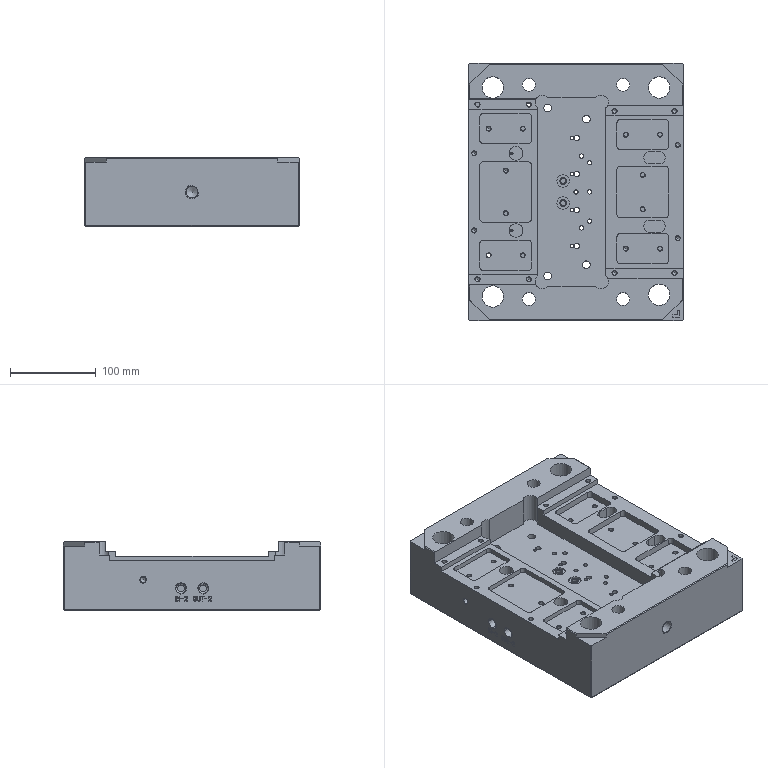CAM job | PowerMill | 3-axis milling, drilling | part box 250 x 300 x 80 mm | stock box 250 x 300 x 80 mm
Tools:
number,name,type,diameter,tip_radius,length,cutting_length,overhang,flutes,holder,toolpaths_using
0,￠10中心钻_1,drill,10.0,0.0,40.0,,10.0,1,D70L70,1
0,￠8中心钻_1,drill,8.0,0.0,40.0,,8.0,1,D70L70,1
0,B21R0.8_1,tip_radiused,21.0,0.8,50.0,,21.0,1,D70L70,1
0,B30R5,tip_radiused,30.0,5.0,50.0,,50.0,1,D70L70,1
0,B30R5_1,tip_radiused,30.0,5.0,50.0,,30.0,1,D70L70,1
0,D3_Q23_1,end_mill,3.0,0.0,30.0,,3.0,1,HSK63-L150-D16,1
0,￠9_1_1,drill,9.0,0.0,40.0,,50.0,1,D35L68,1
0,￠6_1_1,drill,6.0,0.0,40.0,,48.96,1,D35L68,1
0,￠5_1_1,drill,5.0,0.0,40.0,,48.6,1,D35L68,1
0,￠4_1_1,drill,4.0,0.0,40.0,,48.2,1,D35L68,1
0,B17R0.8_1_1,tip_radiused,17.0,0.8,50.0,,40.16,1,D70L70,1
0,D8_1_1,end_mill,8.0,0.0,60.0,,9.24,1,D35L68,1
0,D10_1_1,end_mill,10.0,0.0,75.0,,29.04,1,D50L68,4
0,D6_1_1,end_mill,6.0,0.0,50.0,,14.2,1,D35L68,1
0,B17R0.8_2_1,tip_radiused,17.0,0.8,50.0,,27.76,1,D70L70,1
0,D6_2_1,end_mill,6.0,0.0,50.0,,34.72,1,D35L68,1
0,￠6中心钻_Q17_1_1,drill,6.0,0.0,40.0,,17.76,1,HSK63-L150-D16,1
0,￠4中心钻_1_1,drill,4.0,0.0,40.0,,17.28,1,D70L70,1
0,￠6_2_1,drill,6.0,0.0,40.0,,19.36,1,D35L68,1
0,￠5_2_1,drill,5.0,0.0,40.0,,27.24,1,D35L68,1
0,￠5_3_1,drill,5.0,0.0,40.0,,31.76,1,D35L68,1
0,￠2_1_1,drill,2.0,0.0,40.0,,23.4,1,D35L68,1
0,￠8中心钻_2_1_1,drill,8.0,0.0,40.0,,24.48,1,D70L70,3
Operations:
program,toolpath,strategy,tool,tool_number,tool_diameter,tip_radius,flutes,spindle_rpm,feed_cut,surface_speed_m_min_computed,feed_per_tooth_computed,tolerance,thickness,stepover,stepdown,cut_length,cut_time_min,total_time_min,workplane
005-BA-1,01开粗-￠10中心钻-打中心点,drill,￠10中心钻_1,0,10.0,0.0,1.0,3000.0,60.0,94.25,0.02,0.02,0.0,5.0,1.0,72.0,1.2,1.313,1
005-BA-2,03开粗-￠9-钻孔加工,drill,￠9_1_1,0,9.0,0.0,1.0,600.0,80.0,16.96,0.1333,0.02,0.0,5.0,1.0,281.405,3.518,3.917,1
005-BA-3,04开粗-￠6-钻孔加工,drill,￠6_1_1,0,6.0,0.0,1.0,700.0,80.0,13.19,0.1143,0.02,0.0,5.0,1.0,277.237,3.466,3.96,1
005-BA-4,30开粗-￠5-钻孔加工,drill,￠5_1_1,0,5.0,0.0,1.0,700.0,80.0,11.0,0.1143,0.02,0.0,5.0,1.0,413.648,5.171,5.905,1
005-BA-5,31开粗-￠4-钻孔加工,drill,￠4_1_1,0,4.0,0.0,1.0,800.0,60.0,10.05,0.075,0.02,0.0,5.0,1.0,274.223,4.57,5.282,1
005-BA-6,06中光-B17R0.8-等高,constantz,B17R0.8_1_1,0,17.0,0.8,1.0,2200.0,4000.0,117.5,1.818,0.02,0.1,5.0,0.2,39884.762,9.971,10.052,1
005-BA-7,07中光-D8-等高,constantz,D8_1_1,0,8.0,0.0,1.0,3500.0,3500.0,87.96,1.0,0.01,0.0,5.0,0.18,3914.542,1.118,1.169,1
005-BA-8,11精光-￠8中心钻-倒角,chamfer,￠8中心钻_1,0,8.0,0.0,1.0,4000.0,800.0,100.53,0.2,0.01,0.0,0.18,2.0,364.425,0.456,0.5443,1
005-BB-1,05中光-B21R0.8-等高,constantz,B21R0.8_1,0,21.0,0.8,1.0,2200.0,4500.0,145.14,2.046,0.01,0.0,5.0,0.2,5293.971,1.176,1.595,2
005-BB-2,12开粗-B30R5-偏置区域清除,offset_area_clear,B30R5_1,0,30.0,5.0,1.0,1700.0,4500.0,160.22,2.647,0.01,0.25,16.0,1.0,120912.51,26.869,28.854,2
005-BB-3,13开粗-D10-偏置区域二粗,offset_area_clear,D10_1_1,0,10.0,0.0,1.0,3200.0,5500.0,100.53,1.719,0.02,0.26,6.0,1.0,78250.954,14.228,20.848,2
005-BB-4,32中光-D6-等高,constantz,D6_1_1,0,6.0,0.0,1.0,3800.0,5000.0,71.63,1.316,0.02,0.0,5.0,0.2,2433.87,0.487,1.512,2
005-BB-5,15精光-B17R0.8-偏置平坦面,offset_area_clear,B17R0.8_2_1,0,17.0,0.8,1.0,2200.0,600.0,117.5,0.2727,0.01,0.5,11.0,1.0,5006.723,8.345,8.829,2
005-BB-6,41精光-D10-偏置平坦面,offset_flat,D10_1_1,0,10.0,0.0,1.0,4500.0,1000.0,141.37,0.2222,0.01,0.5,5.0,1.0,95.108,0.095,0.2034,2
005-BB-6,16中光-D10-外形侧光,profile_area_clear,D10_1_1,0,10.0,0.0,1.0,3500.0,1000.0,109.96,0.2857,0.01,0.03,0.05,1.0,3874.063,3.874,4.733,2
005-BB-7,20精光-D10-等高,constantz,D10_1_1,0,10.0,0.0,1.0,5000.0,800.0,157.08,0.16,0.005,-0.02,5.0,18.0,1914.477,2.393,2.808,2
005-BB-8,38精光-D6-等高,constantz,D6_2_1,0,6.0,0.0,1.0,6500.0,2500.0,122.52,0.3846,0.01,0.0,5.0,0.05,12852.384,5.141,7.272,2
005-BB-9,24开粗-￠6中心钻-打中心点,drill,￠6中心钻_Q17_1_1,0,6.0,0.0,1.0,2500.0,60.0,47.12,0.024,0.02,0.0,5.0,1.0,104.0,1.733,2.063,2
005-BB-10,39开粗-￠4中心钻-打中心点,drill,￠4中心钻_1_1,0,4.0,0.0,1.0,3000.0,60.0,37.7,0.02,0.02,0.0,5.0,1.0,8.0,0.133,0.165,2
005-BB-11,25开粗-￠6-钻孔加工,drill,￠6_2_1,0,6.0,0.0,1.0,700.0,80.0,13.19,0.1143,0.02,0.0,5.0,1.0,57.373,0.717,0.7807,2
005-BB-12,34开粗-￠5-钻孔加工,drill,￠5_2_1,0,5.0,0.0,1.0,700.0,80.0,11.0,0.1143,0.02,0.0,5.0,1.0,296.54,3.707,4.033,2
005-BB-13,40开粗-￠5-钻孔加工,drill,￠5_3_1,0,5.0,0.0,1.0,700.0,80.0,11.0,0.1143,0.02,0.0,5.0,1.0,299.54,3.744,4.067,2
005-BB-14,26开粗-￠2-钻孔加工,drill,￠2_1_1,0,2.0,0.0,1.0,1000.0,40.0,6.28,0.04,0.02,0.0,5.0,1.0,31.901,0.797,0.8653,2
005-BB-15,27中光-D3-等高,constantz,D3_Q23_1,0,3.0,0.0,1.0,6500.0,3000.0,61.26,0.4615,0.01,0.0,5.0,0.1,2554.482,0.852,1.127,2
005-BB-16,28精光-￠8中心钻-倒角,chamfer,￠8中心钻_2_1_1,0,8.0,0.0,1.0,4500.0,800.0,113.1,0.1778,0.01,0.0,0.05,2.0,328.169,0.41,0.4902,2
005-BB-16,37精光-￠8中心钻-倒角,chamfer,￠8中心钻_2_1_1,0,8.0,0.0,1.0,4500.0,800.0,113.1,0.1778,0.01,0.0,0.05,2.0,673.789,0.842,0.9357,2
005-BB-16,42精光-￠8中心钻-倒角,chamfer,￠8中心钻_2_1_1,0,8.0,0.0,1.0,4500.0,800.0,113.1,0.1778,0.01,0.0,0.05,2.0,662.503,0.828,0.9188,2
,12开粗-B30R5-偏置区域清除_Reference,offset_area_clear,B30R5,0,30.0,5.0,1.0,1700.0,4500.0,160.22,2.647,0.01,0.25,16.0,1.0,325811.947,72.403,76.8,2